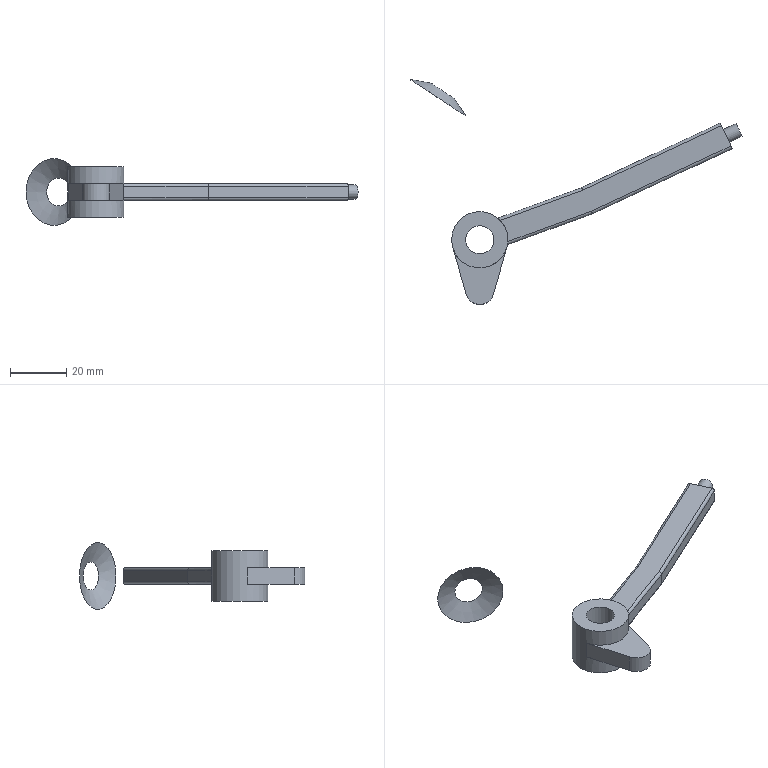Part | NX | features DATUM_CSYS 4, EXTRUDE 3, SKETCH 3, CYLINDER 2, BLEND 1, CPROJ 1, LINKED_FACE 1 | 1 solid | 27 faces | box 117.805 x 79.875 x 23.68 mm | volume 8790 mm3 | plane 14 | cylinder 12 | cone 1 | commonest cylinder face diameters 2 x8 10 x2 5 x1 20 x1